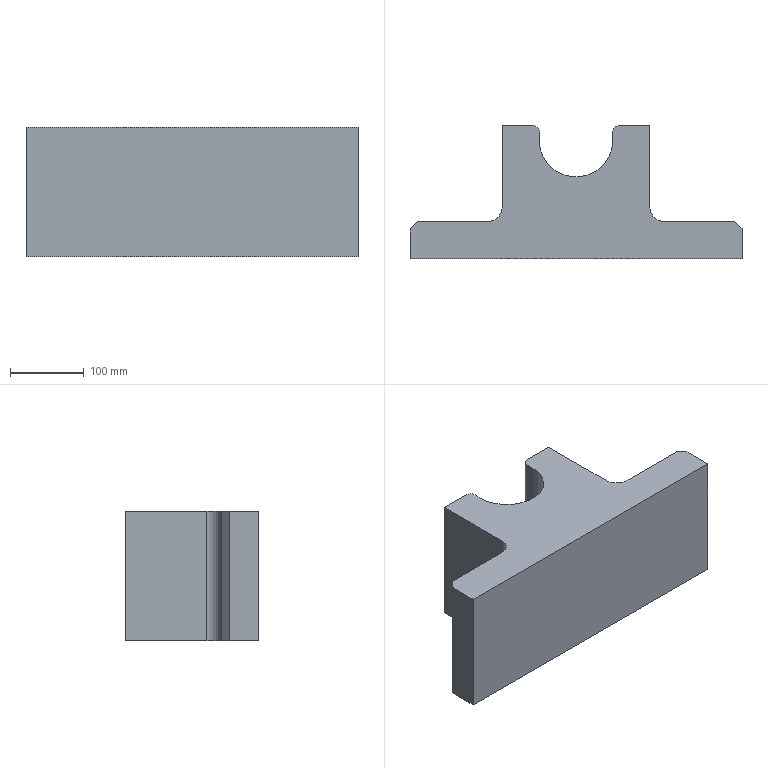Part | SolidWorks | features Fillet 2, Chamfer 1, Extrusion 1, ICE 1, MoveFace 1 | 1 solid | 21 faces | box 450 x 180.5 x 175 mm | volume 7476887 mm3 | plane 13 | cylinder 8 | commonest cylinder face diameters 20 x3 100 x3 40 x2
STEP:
#1=CARTESIAN_POINT('',(49.161,10.,87.5));
#2=VERTEX_POINT('',#1);
#3=CARTESIAN_POINT('',(49.301,8.333,87.5));
#4=VERTEX_POINT('',#3);
#5=CARTESIAN_POINT('',(59.161,10.,87.5));
#6=DIRECTION('',(0.,0.,1.));
#7=DIRECTION('',(1.,0.,0.));
#8=AXIS2_PLACEMENT_3D('',#5,#6,#7);
#9=CIRCLE('',#8,10.);
#10=EDGE_CURVE('',#2,#4,#9,.T.);
#11=ORIENTED_EDGE('',*,*,#10,.F.);
#12=CARTESIAN_POINT('',(49.161,10.,-87.5));
#13=VERTEX_POINT('',#12);
#14=CARTESIAN_POINT('',(49.161,10.,87.5));
#15=DIRECTION('',(0.,0.,-1.));
#16=VECTOR('',#15,1000.);
#17=LINE('',#14,#16);
#18=EDGE_CURVE('',#2,#13,#17,.T.);
#19=ORIENTED_EDGE('',*,*,#18,.T.);
#20=CARTESIAN_POINT('',(49.301,8.333,-87.5));
#21=VERTEX_POINT('',#20);
#22=CARTESIAN_POINT('',(59.161,10.,-87.5));
#23=DIRECTION('',(0.,0.,-1.));
#24=DIRECTION('',(1.,0.,0.));
#25=AXIS2_PLACEMENT_3D('',#22,#23,#24);
#26=CIRCLE('',#25,10.);
#27=EDGE_CURVE('',#21,#13,#26,.T.);
#28=ORIENTED_EDGE('',*,*,#27,.F.);
#29=CARTESIAN_POINT('',(49.301,8.333,87.5));
#30=DIRECTION('',(0.,0.,-1.));
#31=VECTOR('',#30,1000.);
#32=LINE('',#29,#31);
#33=EDGE_CURVE('',#4,#21,#32,.T.);
#34=ORIENTED_EDGE('',*,*,#33,.F.);
#35=EDGE_LOOP('',(#11,#19,#28,#34));
#36=FACE_OUTER_BOUND('',#35,.T.);
#37=CARTESIAN_POINT('',(59.161,10.,87.5));
#38=DIRECTION('',(0.,0.,-1.));
#39=DIRECTION('',(-1.,0.,0.));
#40=AXIS2_PLACEMENT_3D('',#37,#38,#39);
#41=CYLINDRICAL_SURFACE('',#40,10.);
#42=ADVANCED_FACE('',(#36),#41,.T.);
#43=CARTESIAN_POINT('',(-50.,0.,87.5));
#44=VERTEX_POINT('',#43);
#45=CARTESIAN_POINT('',(50.,0.,87.5));
#46=VERTEX_POINT('',#45);
#47=CARTESIAN_POINT('',(0.,0.,87.5));
#48=DIRECTION('',(0.,0.,1.));
#49=DIRECTION('',(1.,0.,0.));
#50=AXIS2_PLACEMENT_3D('',#47,#48,#49);
#51=CIRCLE('',#50,50.);
#52=EDGE_CURVE('',#44,#46,#51,.T.);
#53=ORIENTED_EDGE('',*,*,#52,.T.);
#54=CARTESIAN_POINT('',(50.,0.,-87.5));
#55=VERTEX_POINT('',#54);
#56=CARTESIAN_POINT('',(50.,0.,87.5));
#57=DIRECTION('',(0.,0.,-1.));
#58=VECTOR('',#57,1000.);
#59=LINE('',#56,#58);
#60=EDGE_CURVE('',#46,#55,#59,.T.);
#61=ORIENTED_EDGE('',*,*,#60,.T.);
#62=CARTESIAN_POINT('',(-50.,0.,-87.5));
#63=VERTEX_POINT('',#62);
#64=CARTESIAN_POINT('',(0.,0.,-87.5));
#65=DIRECTION('',(0.,0.,1.));
#66=DIRECTION('',(1.,0.,0.));
#67=AXIS2_PLACEMENT_3D('',#64,#65,#66);
#68=CIRCLE('',#67,50.);
#69=EDGE_CURVE('',#63,#55,#68,.T.);
#70=ORIENTED_EDGE('',*,*,#69,.F.);
#71=CARTESIAN_POINT('',(-50.,0.,87.5));
#72=DIRECTION('',(0.,0.,-1.));
#73=VECTOR('',#72,1000.);
#74=LINE('',#71,#73);
#75=EDGE_CURVE('',#44,#63,#74,.T.);
#76=ORIENTED_EDGE('',*,*,#75,.F.);
#77=EDGE_LOOP('',(#53,#61,#70,#76));
#78=FACE_OUTER_BOUND('',#77,.T.);
#79=CARTESIAN_POINT('',(0.,0.,87.5));
#80=DIRECTION('',(0.,0.,-1.));
#81=DIRECTION('',(-1.,0.,0.));
#82=AXIS2_PLACEMENT_3D('',#79,#80,#81);
#83=CYLINDRICAL_SURFACE('',#82,50.);
#84=ADVANCED_FACE('',(#78),#83,.F.);
#85=CARTESIAN_POINT('',(-49.301,8.333,87.5));
#86=VERTEX_POINT('',#85);
#87=CARTESIAN_POINT('',(0.,0.,87.5));
#88=DIRECTION('',(0.,0.,1.));
#89=DIRECTION('',(1.,0.,0.));
#90=AXIS2_PLACEMENT_3D('',#87,#88,#89);
#91=CIRCLE('',#90,50.);
#92=EDGE_CURVE('',#86,#44,#91,.T.);
#93=ORIENTED_EDGE('',*,*,#92,.T.);
#94=ORIENTED_EDGE('',*,*,#75,.T.);
#95=CARTESIAN_POINT('',(-49.301,8.333,-87.5));
#96=VERTEX_POINT('',#95);
#97=CARTESIAN_POINT('',(0.,0.,-87.5));
#98=DIRECTION('',(0.,0.,1.));
#99=DIRECTION('',(1.,0.,0.));
#100=AXIS2_PLACEMENT_3D('',#97,#98,#99);
#101=CIRCLE('',#100,50.);
#102=EDGE_CURVE('',#96,#63,#101,.T.);
#103=ORIENTED_EDGE('',*,*,#102,.F.);
#104=CARTESIAN_POINT('',(-49.301,8.333,87.5));
#105=DIRECTION('',(0.,0.,1.));
#106=VECTOR('',#105,1000.);
#107=LINE('',#104,#106);
#108=EDGE_CURVE('',#96,#86,#107,.T.);
#109=ORIENTED_EDGE('',*,*,#108,.T.);
#110=EDGE_LOOP('',(#93,#94,#103,#109));
#111=FACE_OUTER_BOUND('',#110,.T.);
#112=CARTESIAN_POINT('',(0.,0.,87.5));
#113=DIRECTION('',(0.,0.,-1.));
#114=DIRECTION('',(-1.,0.,0.));
#115=AXIS2_PLACEMENT_3D('',#112,#113,#114);
#116=CYLINDRICAL_SURFACE('',#115,50.);
#117=ADVANCED_FACE('',(#111),#116,.F.);
#118=ORIENTED_EDGE('',*,*,#60,.F.);
#119=CARTESIAN_POINT('',(0.,0.,87.5));
#120=DIRECTION('',(0.,0.,1.));
#121=DIRECTION('',(1.,0.,0.));
#122=AXIS2_PLACEMENT_3D('',#119,#120,#121);
#123=CIRCLE('',#122,50.);
#124=EDGE_CURVE('',#46,#4,#123,.T.);
#125=ORIENTED_EDGE('',*,*,#124,.T.);
#126=ORIENTED_EDGE('',*,*,#33,.T.);
#127=CARTESIAN_POINT('',(0.,0.,-87.5));
#128=DIRECTION('',(0.,0.,1.));
#129=DIRECTION('',(1.,0.,0.));
#130=AXIS2_PLACEMENT_3D('',#127,#128,#129);
#131=CIRCLE('',#130,50.);
#132=EDGE_CURVE('',#55,#21,#131,.T.);
#133=ORIENTED_EDGE('',*,*,#132,.F.);
#134=EDGE_LOOP('',(#118,#125,#126,#133));
#135=FACE_OUTER_BOUND('',#134,.T.);
#136=CARTESIAN_POINT('',(0.,0.,87.5));
#137=DIRECTION('',(0.,0.,-1.));
#138=DIRECTION('',(-1.,0.,0.));
#139=AXIS2_PLACEMENT_3D('',#136,#137,#138);
#140=CYLINDRICAL_SURFACE('',#139,50.);
#141=ADVANCED_FACE('',(#135),#140,.F.);
#142=CARTESIAN_POINT('',(225.,-120.5,87.5));
#143=VERTEX_POINT('',#142);
#144=CARTESIAN_POINT('',(225.,-160.5,87.5));
#145=VERTEX_POINT('',#144);
#146=CARTESIAN_POINT('',(225.,0.,87.5));
#147=DIRECTION('',(0.,-1.,0.));
#148=VECTOR('',#147,1000.);
#149=LINE('',#146,#148);
#150=EDGE_CURVE('',#143,#145,#149,.T.);
#151=ORIENTED_EDGE('',*,*,#150,.F.);
#152=CARTESIAN_POINT('',(215.,-110.5,87.5));
#153=VERTEX_POINT('',#152);
#154=CARTESIAN_POINT('',(52.25,52.25,87.5));
#155=DIRECTION('',(-0.7071,0.7071,0.));
#156=VECTOR('',#155,1000.);
#157=LINE('',#154,#156);
#158=EDGE_CURVE('',#143,#153,#157,.T.);
#159=ORIENTED_EDGE('',*,*,#158,.T.);
#160=CARTESIAN_POINT('',(120.,-110.5,87.5));
#161=VERTEX_POINT('',#160);
#162=CARTESIAN_POINT('',(0.,-110.5,87.5));
#163=DIRECTION('',(1.,0.,0.));
#164=VECTOR('',#163,1000.);
#165=LINE('',#162,#164);
#166=EDGE_CURVE('',#161,#153,#165,.T.);
#167=ORIENTED_EDGE('',*,*,#166,.F.);
#168=CARTESIAN_POINT('',(100.,-90.5,87.5));
#169=VERTEX_POINT('',#168);
#170=CARTESIAN_POINT('',(120.,-90.5,87.5));
#171=DIRECTION('',(0.,0.,-1.));
#172=DIRECTION('',(1.,0.,0.));
#173=AXIS2_PLACEMENT_3D('',#170,#171,#172);
#174=CIRCLE('',#173,20.);
#175=EDGE_CURVE('',#161,#169,#174,.T.);
#176=ORIENTED_EDGE('',*,*,#175,.T.);
#177=CARTESIAN_POINT('',(100.,20.,87.5));
#178=VERTEX_POINT('',#177);
#179=CARTESIAN_POINT('',(100.,0.,87.5));
#180=DIRECTION('',(0.,1.,0.));
#181=VECTOR('',#180,1000.);
#182=LINE('',#179,#181);
#183=EDGE_CURVE('',#169,#178,#182,.T.);
#184=ORIENTED_EDGE('',*,*,#183,.T.);
#185=CARTESIAN_POINT('',(59.161,20.,87.5));
#186=VERTEX_POINT('',#185);
#187=CARTESIAN_POINT('',(-100.,20.,87.5));
#188=DIRECTION('',(1.,0.,0.));
#189=VECTOR('',#188,1000.);
#190=LINE('',#187,#189);
#191=EDGE_CURVE('',#186,#178,#190,.T.);
#192=ORIENTED_EDGE('',*,*,#191,.F.);
#193=CARTESIAN_POINT('',(59.161,10.,87.5));
#194=DIRECTION('',(0.,0.,1.));
#195=DIRECTION('',(1.,0.,0.));
#196=AXIS2_PLACEMENT_3D('',#193,#194,#195);
#197=CIRCLE('',#196,10.);
#198=EDGE_CURVE('',#186,#2,#197,.T.);
#199=ORIENTED_EDGE('',*,*,#198,.T.);
#200=ORIENTED_EDGE('',*,*,#10,.T.);
#201=ORIENTED_EDGE('',*,*,#124,.F.);
#202=ORIENTED_EDGE('',*,*,#52,.F.);
#203=ORIENTED_EDGE('',*,*,#92,.F.);
#204=CARTESIAN_POINT('',(-59.161,20.,87.5));
#205=VERTEX_POINT('',#204);
#206=CARTESIAN_POINT('',(-59.161,10.,87.5));
#207=DIRECTION('',(0.,0.,1.));
#208=DIRECTION('',(1.,0.,0.));
#209=AXIS2_PLACEMENT_3D('',#206,#207,#208);
#210=CIRCLE('',#209,10.);
#211=EDGE_CURVE('',#86,#205,#210,.T.);
#212=ORIENTED_EDGE('',*,*,#211,.T.);
#213=CARTESIAN_POINT('',(-100.,20.,87.5));
#214=VERTEX_POINT('',#213);
#215=CARTESIAN_POINT('',(-100.,20.,87.5));
#216=DIRECTION('',(1.,0.,0.));
#217=VECTOR('',#216,1000.);
#218=LINE('',#215,#217);
#219=EDGE_CURVE('',#214,#205,#218,.T.);
#220=ORIENTED_EDGE('',*,*,#219,.F.);
#221=CARTESIAN_POINT('',(-100.,-90.5,87.5));
#222=VERTEX_POINT('',#221);
#223=CARTESIAN_POINT('',(-100.,0.,87.5));
#224=DIRECTION('',(0.,1.,0.));
#225=VECTOR('',#224,1000.);
#226=LINE('',#223,#225);
#227=EDGE_CURVE('',#222,#214,#226,.T.);
#228=ORIENTED_EDGE('',*,*,#227,.F.);
#229=CARTESIAN_POINT('',(-120.,-110.5,87.5));
#230=VERTEX_POINT('',#229);
#231=CARTESIAN_POINT('',(-120.,-90.5,87.5));
#232=DIRECTION('',(0.,0.,-1.));
#233=DIRECTION('',(1.,0.,0.));
#234=AXIS2_PLACEMENT_3D('',#231,#232,#233);
#235=CIRCLE('',#234,20.);
#236=EDGE_CURVE('',#222,#230,#235,.T.);
#237=ORIENTED_EDGE('',*,*,#236,.T.);
#238=CARTESIAN_POINT('',(-215.,-110.5,87.5));
#239=VERTEX_POINT('',#238);
#240=CARTESIAN_POINT('',(0.,-110.5,87.5));
#241=DIRECTION('',(1.,0.,0.));
#242=VECTOR('',#241,1000.);
#243=LINE('',#240,#242);
#244=EDGE_CURVE('',#239,#230,#243,.T.);
#245=ORIENTED_EDGE('',*,*,#244,.F.);
#246=CARTESIAN_POINT('',(-225.,-120.5,87.5));
#247=VERTEX_POINT('',#246);
#248=CARTESIAN_POINT('',(-52.25,52.25,87.5));
#249=DIRECTION('',(-0.7071,-0.7071,0.));
#250=VECTOR('',#249,1000.);
#251=LINE('',#248,#250);
#252=EDGE_CURVE('',#239,#247,#251,.T.);
#253=ORIENTED_EDGE('',*,*,#252,.T.);
#254=CARTESIAN_POINT('',(-225.,-160.5,87.5));
#255=VERTEX_POINT('',#254);
#256=CARTESIAN_POINT('',(-225.,0.,87.5));
#257=DIRECTION('',(0.,-1.,0.));
#258=VECTOR('',#257,1000.);
#259=LINE('',#256,#258);
#260=EDGE_CURVE('',#247,#255,#259,.T.);
#261=ORIENTED_EDGE('',*,*,#260,.T.);
#262=CARTESIAN_POINT('',(0.,-160.5,87.5));
#263=DIRECTION('',(1.,0.,0.));
#264=VECTOR('',#263,1000.);
#265=LINE('',#262,#264);
#266=EDGE_CURVE('',#255,#145,#265,.T.);
#267=ORIENTED_EDGE('',*,*,#266,.T.);
#268=EDGE_LOOP('',(#151,#159,#167,#176,#184,#192,#199,#200,#201,#202,#203,#212,#220,#228,#237,#245,#253,#261,#267));
#269=FACE_OUTER_BOUND('',#268,.T.);
#270=CARTESIAN_POINT('',(0.,0.,87.5));
#271=DIRECTION('',(0.,0.,1.));
#272=DIRECTION('',(1.,0.,0.));
#273=AXIS2_PLACEMENT_3D('',#270,#271,#272);
#274=PLANE('',#273);
#275=ADVANCED_FACE('',(#269),#274,.T.);
#276=CARTESIAN_POINT('',(120.,-110.5,-87.5));
#277=VERTEX_POINT('',#276);
#278=CARTESIAN_POINT('',(215.,-110.5,-87.5));
#279=VERTEX_POINT('',#278);
#280=CARTESIAN_POINT('',(0.,-110.5,-87.5));
#281=DIRECTION('',(1.,0.,0.));
#282=VECTOR('',#281,1000.);
#283=LINE('',#280,#282);
#284=EDGE_CURVE('',#277,#279,#283,.T.);
#285=ORIENTED_EDGE('',*,*,#284,.T.);
#286=CARTESIAN_POINT('',(225.,-120.5,-87.5));
#287=VERTEX_POINT('',#286);
#288=CARTESIAN_POINT('',(215.,-110.5,-87.5));
#289=DIRECTION('',(0.7071,-0.7071,0.));
#290=VECTOR('',#289,1000.);
#291=LINE('',#288,#290);
#292=EDGE_CURVE('',#279,#287,#291,.T.);
#293=ORIENTED_EDGE('',*,*,#292,.T.);
#294=CARTESIAN_POINT('',(225.,-160.5,-87.5));
#295=VERTEX_POINT('',#294);
#296=CARTESIAN_POINT('',(225.,0.,-87.5));
#297=DIRECTION('',(0.,-1.,0.));
#298=VECTOR('',#297,1000.);
#299=LINE('',#296,#298);
#300=EDGE_CURVE('',#287,#295,#299,.T.);
#301=ORIENTED_EDGE('',*,*,#300,.T.);
#302=CARTESIAN_POINT('',(-225.,-160.5,-87.5));
#303=VERTEX_POINT('',#302);
#304=CARTESIAN_POINT('',(0.,-160.5,-87.5));
#305=DIRECTION('',(1.,0.,0.));
#306=VECTOR('',#305,1000.);
#307=LINE('',#304,#306);
#308=EDGE_CURVE('',#303,#295,#307,.T.);
#309=ORIENTED_EDGE('',*,*,#308,.F.);
#310=CARTESIAN_POINT('',(-225.,-120.5,-87.5));
#311=VERTEX_POINT('',#310);
#312=CARTESIAN_POINT('',(-225.,0.,-87.5));
#313=DIRECTION('',(0.,-1.,0.));
#314=VECTOR('',#313,1000.);
#315=LINE('',#312,#314);
#316=EDGE_CURVE('',#311,#303,#315,.T.);
#317=ORIENTED_EDGE('',*,*,#316,.F.);
#318=CARTESIAN_POINT('',(-215.,-110.5,-87.5));
#319=VERTEX_POINT('',#318);
#320=CARTESIAN_POINT('',(-225.,-120.5,-87.5));
#321=DIRECTION('',(0.7071,0.7071,0.));
#322=VECTOR('',#321,1000.);
#323=LINE('',#320,#322);
#324=EDGE_CURVE('',#311,#319,#323,.T.);
#325=ORIENTED_EDGE('',*,*,#324,.T.);
#326=CARTESIAN_POINT('',(-120.,-110.5,-87.5));
#327=VERTEX_POINT('',#326);
#328=CARTESIAN_POINT('',(0.,-110.5,-87.5));
#329=DIRECTION('',(1.,0.,0.));
#330=VECTOR('',#329,1000.);
#331=LINE('',#328,#330);
#332=EDGE_CURVE('',#319,#327,#331,.T.);
#333=ORIENTED_EDGE('',*,*,#332,.T.);
#334=CARTESIAN_POINT('',(-100.,-90.5,-87.5));
#335=VERTEX_POINT('',#334);
#336=CARTESIAN_POINT('',(-120.,-90.5,-87.5));
#337=DIRECTION('',(0.,0.,1.));
#338=DIRECTION('',(1.,0.,0.));
#339=AXIS2_PLACEMENT_3D('',#336,#337,#338);
#340=CIRCLE('',#339,20.);
#341=EDGE_CURVE('',#327,#335,#340,.T.);
#342=ORIENTED_EDGE('',*,*,#341,.T.);
#343=CARTESIAN_POINT('',(-100.,20.,-87.5));
#344=VERTEX_POINT('',#343);
#345=CARTESIAN_POINT('',(-100.,0.,-87.5));
#346=DIRECTION('',(0.,1.,0.));
#347=VECTOR('',#346,1000.);
#348=LINE('',#345,#347);
#349=EDGE_CURVE('',#335,#344,#348,.T.);
#350=ORIENTED_EDGE('',*,*,#349,.T.);
#351=CARTESIAN_POINT('',(-59.161,20.,-87.5));
#352=VERTEX_POINT('',#351);
#353=CARTESIAN_POINT('',(0.,20.,-87.5));
#354=DIRECTION('',(-1.,0.,0.));
#355=VECTOR('',#354,1000.);
#356=LINE('',#353,#355);
#357=EDGE_CURVE('',#352,#344,#356,.T.);
#358=ORIENTED_EDGE('',*,*,#357,.F.);
#359=CARTESIAN_POINT('',(-59.161,10.,-87.5));
#360=DIRECTION('',(0.,0.,-1.));
#361=DIRECTION('',(1.,0.,0.));
#362=AXIS2_PLACEMENT_3D('',#359,#360,#361);
#363=CIRCLE('',#362,10.);
#364=EDGE_CURVE('',#352,#96,#363,.T.);
#365=ORIENTED_EDGE('',*,*,#364,.T.);
#366=ORIENTED_EDGE('',*,*,#102,.T.);
#367=ORIENTED_EDGE('',*,*,#69,.T.);
#368=ORIENTED_EDGE('',*,*,#132,.T.);
#369=ORIENTED_EDGE('',*,*,#27,.T.);
#370=CARTESIAN_POINT('',(59.161,20.,-87.5));
#371=VERTEX_POINT('',#370);
#372=CARTESIAN_POINT('',(59.161,10.,-87.5));
#373=DIRECTION('',(0.,0.,-1.));
#374=DIRECTION('',(1.,0.,0.));
#375=AXIS2_PLACEMENT_3D('',#372,#373,#374);
#376=CIRCLE('',#375,10.);
#377=EDGE_CURVE('',#13,#371,#376,.T.);
#378=ORIENTED_EDGE('',*,*,#377,.T.);
#379=CARTESIAN_POINT('',(100.,20.,-87.5));
#380=VERTEX_POINT('',#379);
#381=CARTESIAN_POINT('',(-100.,20.,-87.5));
#382=DIRECTION('',(-1.,0.,0.));
#383=VECTOR('',#382,1000.);
#384=LINE('',#381,#383);
#385=EDGE_CURVE('',#380,#371,#384,.T.);
#386=ORIENTED_EDGE('',*,*,#385,.F.);
#387=CARTESIAN_POINT('',(100.,-90.5,-87.5));
#388=VERTEX_POINT('',#387);
#389=CARTESIAN_POINT('',(100.,0.,-87.5));
#390=DIRECTION('',(0.,1.,0.));
#391=VECTOR('',#390,1000.);
#392=LINE('',#389,#391);
#393=EDGE_CURVE('',#388,#380,#392,.T.);
#394=ORIENTED_EDGE('',*,*,#393,.F.);
#395=CARTESIAN_POINT('',(120.,-90.5,-87.5));
#396=DIRECTION('',(0.,0.,1.));
#397=DIRECTION('',(1.,0.,0.));
#398=AXIS2_PLACEMENT_3D('',#395,#396,#397);
#399=CIRCLE('',#398,20.);
#400=EDGE_CURVE('',#388,#277,#399,.T.);
#401=ORIENTED_EDGE('',*,*,#400,.T.);
#402=EDGE_LOOP('',(#285,#293,#301,#309,#317,#325,#333,#342,#350,#358,#365,#366,#367,#368,#369,#378,#386,#394,#401));
#403=FACE_OUTER_BOUND('',#402,.T.);
#404=CARTESIAN_POINT('',(0.,0.,-87.5));
#405=DIRECTION('',(0.,0.,1.));
#406=DIRECTION('',(1.,0.,0.));
#407=AXIS2_PLACEMENT_3D('',#404,#405,#406);
#408=PLANE('',#407);
#409=ADVANCED_FACE('',(#403),#408,.F.);
#410=ORIENTED_EDGE('',*,*,#183,.F.);
#411=CARTESIAN_POINT('',(100.,-90.5,87.5));
#412=DIRECTION('',(0.,0.,-1.));
#413=VECTOR('',#412,1000.);
#414=LINE('',#411,#413);
#415=EDGE_CURVE('',#169,#388,#414,.T.);
#416=ORIENTED_EDGE('',*,*,#415,.T.);
#417=ORIENTED_EDGE('',*,*,#393,.T.);
#418=CARTESIAN_POINT('',(100.,20.,87.5));
#419=DIRECTION('',(0.,0.,-1.));
#420=VECTOR('',#419,1000.);
#421=LINE('',#418,#420);
#422=EDGE_CURVE('',#178,#380,#421,.T.);
#423=ORIENTED_EDGE('',*,*,#422,.F.);
#424=EDGE_LOOP('',(#410,#416,#417,#423));
#425=FACE_OUTER_BOUND('',#424,.T.);
#426=CARTESIAN_POINT('',(100.,0.,87.5));
#427=DIRECTION('',(-1.,0.,0.));
#428=DIRECTION('',(0.,-1.,0.));
#429=AXIS2_PLACEMENT_3D('',#426,#427,#428);
#430=PLANE('',#429);
#431=ADVANCED_FACE('',(#425),#430,.F.);
#432=ORIENTED_EDGE('',*,*,#349,.F.);
#433=CARTESIAN_POINT('',(-100.,-90.5,87.5));
#434=DIRECTION('',(0.,0.,1.));
#435=VECTOR('',#434,1000.);
#436=LINE('',#433,#435);
#437=EDGE_CURVE('',#335,#222,#436,.T.);
#438=ORIENTED_EDGE('',*,*,#437,.T.);
#439=ORIENTED_EDGE('',*,*,#227,.T.);
#440=CARTESIAN_POINT('',(-100.,20.,87.5));
#441=DIRECTION('',(0.,0.,-1.));
#442=VECTOR('',#441,1000.);
#443=LINE('',#440,#442);
#444=EDGE_CURVE('',#214,#344,#443,.T.);
#445=ORIENTED_EDGE('',*,*,#444,.T.);
#446=EDGE_LOOP('',(#432,#438,#439,#445));
#447=FACE_OUTER_BOUND('',#446,.T.);
#448=CARTESIAN_POINT('',(-100.,0.,87.5));
#449=DIRECTION('',(-1.,0.,0.));
#450=DIRECTION('',(0.,-1.,0.));
#451=AXIS2_PLACEMENT_3D('',#448,#449,#450);
#452=PLANE('',#451);
#453=ADVANCED_FACE('',(#447),#452,.T.);
#454=ORIENTED_EDGE('',*,*,#332,.F.);
#455=CARTESIAN_POINT('',(-215.,-110.5,87.5));
#456=DIRECTION('',(0.,0.,1.));
#457=VECTOR('',#456,1000.);
#458=LINE('',#455,#457);
#459=EDGE_CURVE('',#319,#239,#458,.T.);
#460=ORIENTED_EDGE('',*,*,#459,.T.);
#461=ORIENTED_EDGE('',*,*,#244,.T.);
#462=CARTESIAN_POINT('',(-120.,-110.5,-87.5));
#463=DIRECTION('',(0.,0.,-1.));
#464=VECTOR('',#463,1000.);
#465=LINE('',#462,#464);
#466=EDGE_CURVE('',#230,#327,#465,.T.);
#467=ORIENTED_EDGE('',*,*,#466,.T.);
#468=EDGE_LOOP('',(#454,#460,#461,#467));
#469=FACE_OUTER_BOUND('',#468,.T.);
#470=CARTESIAN_POINT('',(0.,-110.5,87.5));
#471=DIRECTION('',(0.,1.,0.));
#472=DIRECTION('',(-1.,0.,0.));
#473=AXIS2_PLACEMENT_3D('',#470,#471,#472);
#474=PLANE('',#473);
#475=ADVANCED_FACE('',(#469),#474,.T.);
#476=ORIENTED_EDGE('',*,*,#260,.F.);
#477=CARTESIAN_POINT('',(-225.,-120.5,-87.5));
#478=DIRECTION('',(0.,0.,-1.));
#479=VECTOR('',#478,1000.);
#480=LINE('',#477,#479);
#481=EDGE_CURVE('',#247,#311,#480,.T.);
#482=ORIENTED_EDGE('',*,*,#481,.T.);
#483=ORIENTED_EDGE('',*,*,#316,.T.);
#484=CARTESIAN_POINT('',(-225.,-160.5,87.5));
#485=DIRECTION('',(0.,0.,-1.));
#486=VECTOR('',#485,1000.);
#487=LINE('',#484,#486);
#488=EDGE_CURVE('',#255,#303,#487,.T.);
#489=ORIENTED_EDGE('',*,*,#488,.F.);
#490=EDGE_LOOP('',(#476,#482,#483,#489));
#491=FACE_OUTER_BOUND('',#490,.T.);
#492=CARTESIAN_POINT('',(-225.,0.,87.5));
#493=DIRECTION('',(1.,0.,0.));
#494=DIRECTION('',(0.,0.,-1.));
#495=AXIS2_PLACEMENT_3D('',#492,#493,#494);
#496=PLANE('',#495);
#497=ADVANCED_FACE('',(#491),#496,.F.);
#498=ORIENTED_EDGE('',*,*,#308,.T.);
#499=CARTESIAN_POINT('',(225.,-160.5,87.5));
#500=DIRECTION('',(0.,0.,-1.));
#501=VECTOR('',#500,1000.);
#502=LINE('',#499,#501);
#503=EDGE_CURVE('',#145,#295,#502,.T.);
#504=ORIENTED_EDGE('',*,*,#503,.F.);
#505=ORIENTED_EDGE('',*,*,#266,.F.);
#506=ORIENTED_EDGE('',*,*,#488,.T.);
#507=EDGE_LOOP('',(#498,#504,#505,#506));
#508=FACE_OUTER_BOUND('',#507,.T.);
#509=CARTESIAN_POINT('',(0.,-160.5,87.5));
#510=DIRECTION('',(0.,1.,0.));
#511=DIRECTION('',(-1.,0.,0.));
#512=AXIS2_PLACEMENT_3D('',#509,#510,#511);
#513=PLANE('',#512);
#514=ADVANCED_FACE('',(#508),#513,.F.);
#515=ORIENTED_EDGE('',*,*,#300,.F.);
#516=CARTESIAN_POINT('',(225.,-120.5,87.5));
#517=DIRECTION('',(0.,0.,1.));
#518=VECTOR('',#517,1000.);
#519=LINE('',#516,#518);
#520=EDGE_CURVE('',#287,#143,#519,.T.);
#521=ORIENTED_EDGE('',*,*,#520,.T.);
#522=ORIENTED_EDGE('',*,*,#150,.T.);
#523=ORIENTED_EDGE('',*,*,#503,.T.);
#524=EDGE_LOOP('',(#515,#521,#522,#523));
#525=FACE_OUTER_BOUND('',#524,.T.);
#526=CARTESIAN_POINT('',(225.,0.,87.5));
#527=DIRECTION('',(1.,0.,0.));
#528=DIRECTION('',(0.,1.,0.));
#529=AXIS2_PLACEMENT_3D('',#526,#527,#528);
#530=PLANE('',#529);
#531=ADVANCED_FACE('',(#525),#530,.T.);
#532=ORIENTED_EDGE('',*,*,#166,.T.);
#533=CARTESIAN_POINT('',(215.,-110.5,87.5));
#534=DIRECTION('',(0.,0.,-1.));
#535=VECTOR('',#534,1000.);
#536=LINE('',#533,#535);
#537=EDGE_CURVE('',#153,#279,#536,.T.);
#538=ORIENTED_EDGE('',*,*,#537,.T.);
#539=ORIENTED_EDGE('',*,*,#284,.F.);
#540=CARTESIAN_POINT('',(120.,-110.5,87.5));
#541=DIRECTION('',(0.,0.,1.));
#542=VECTOR('',#541,1000.);
#543=LINE('',#540,#542);
#544=EDGE_CURVE('',#277,#161,#543,.T.);
#545=ORIENTED_EDGE('',*,*,#544,.T.);
#546=EDGE_LOOP('',(#532,#538,#539,#545));
#547=FACE_OUTER_BOUND('',#546,.T.);
#548=CARTESIAN_POINT('',(0.,-110.5,87.5));
#549=DIRECTION('',(0.,1.,0.));
#550=DIRECTION('',(-1.,0.,0.));
#551=AXIS2_PLACEMENT_3D('',#548,#549,#550);
#552=PLANE('',#551);
#553=ADVANCED_FACE('',(#547),#552,.T.);
#554=ORIENTED_EDGE('',*,*,#219,.T.);
#555=CARTESIAN_POINT('',(-59.161,20.,0.));
#556=DIRECTION('',(0.,0.,-1.));
#557=VECTOR('',#556,1000.);
#558=LINE('',#555,#557);
#559=EDGE_CURVE('',#205,#352,#558,.T.);
#560=ORIENTED_EDGE('',*,*,#559,.T.);
#561=ORIENTED_EDGE('',*,*,#357,.T.);
#562=ORIENTED_EDGE('',*,*,#444,.F.);
#563=EDGE_LOOP('',(#554,#560,#561,#562));
#564=FACE_OUTER_BOUND('',#563,.T.);
#565=CARTESIAN_POINT('',(0.,20.,0.));
#566=DIRECTION('',(0.,1.,0.));
#567=DIRECTION('',(0.,0.,1.));
#568=AXIS2_PLACEMENT_3D('',#565,#566,#567);
#569=PLANE('',#568);
#570=ADVANCED_FACE('',(#564),#569,.T.);
#571=ORIENTED_EDGE('',*,*,#385,.T.);
#572=CARTESIAN_POINT('',(59.161,20.,0.));
#573=DIRECTION('',(0.,0.,1.));
#574=VECTOR('',#573,1000.);
#575=LINE('',#572,#574);
#576=EDGE_CURVE('',#371,#186,#575,.T.);
#577=ORIENTED_EDGE('',*,*,#576,.T.);
#578=ORIENTED_EDGE('',*,*,#191,.T.);
#579=ORIENTED_EDGE('',*,*,#422,.T.);
#580=EDGE_LOOP('',(#571,#577,#578,#579));
#581=FACE_OUTER_BOUND('',#580,.T.);
#582=CARTESIAN_POINT('',(0.,20.,0.));
#583=DIRECTION('',(0.,1.,0.));
#584=DIRECTION('',(0.,0.,1.));
#585=AXIS2_PLACEMENT_3D('',#582,#583,#584);
#586=PLANE('',#585);
#587=ADVANCED_FACE('',(#581),#586,.T.);
#588=ORIENTED_EDGE('',*,*,#18,.F.);
#589=ORIENTED_EDGE('',*,*,#198,.F.);
#590=ORIENTED_EDGE('',*,*,#576,.F.);
#591=ORIENTED_EDGE('',*,*,#377,.F.);
#592=EDGE_LOOP('',(#588,#589,#590,#591));
#593=FACE_OUTER_BOUND('',#592,.T.);
#594=CARTESIAN_POINT('',(59.161,10.,87.5));
#595=DIRECTION('',(0.,0.,-1.));
#596=DIRECTION('',(-1.,0.,0.));
#597=AXIS2_PLACEMENT_3D('',#594,#595,#596);
#598=CYLINDRICAL_SURFACE('',#597,10.);
#599=ADVANCED_FACE('',(#593),#598,.T.);
#600=ORIENTED_EDGE('',*,*,#364,.F.);
#601=ORIENTED_EDGE('',*,*,#559,.F.);
#602=ORIENTED_EDGE('',*,*,#211,.F.);
#603=ORIENTED_EDGE('',*,*,#108,.F.);
#604=EDGE_LOOP('',(#600,#601,#602,#603));
#605=FACE_OUTER_BOUND('',#604,.T.);
#606=CARTESIAN_POINT('',(-59.161,10.,87.5));
#607=DIRECTION('',(0.,0.,-1.));
#608=DIRECTION('',(-1.,0.,0.));
#609=AXIS2_PLACEMENT_3D('',#606,#607,#608);
#610=CYLINDRICAL_SURFACE('',#609,10.);
#611=ADVANCED_FACE('',(#605),#610,.T.);
#612=ORIENTED_EDGE('',*,*,#236,.F.);
#613=ORIENTED_EDGE('',*,*,#437,.F.);
#614=ORIENTED_EDGE('',*,*,#341,.F.);
#615=ORIENTED_EDGE('',*,*,#466,.F.);
#616=EDGE_LOOP('',(#612,#613,#614,#615));
#617=FACE_OUTER_BOUND('',#616,.T.);
#618=CARTESIAN_POINT('',(-120.,-90.5,87.5));
#619=DIRECTION('',(0.,0.,1.));
#620=DIRECTION('',(1.,0.,0.));
#621=AXIS2_PLACEMENT_3D('',#618,#619,#620);
#622=CYLINDRICAL_SURFACE('',#621,20.);
#623=ADVANCED_FACE('',(#617),#622,.F.);
#624=ORIENTED_EDGE('',*,*,#175,.F.);
#625=ORIENTED_EDGE('',*,*,#544,.F.);
#626=ORIENTED_EDGE('',*,*,#400,.F.);
#627=ORIENTED_EDGE('',*,*,#415,.F.);
#628=EDGE_LOOP('',(#624,#625,#626,#627));
#629=FACE_OUTER_BOUND('',#628,.T.);
#630=CARTESIAN_POINT('',(120.,-90.5,87.5));
#631=DIRECTION('',(0.,0.,-1.));
#632=DIRECTION('',(-1.,0.,0.));
#633=AXIS2_PLACEMENT_3D('',#630,#631,#632);
#634=CYLINDRICAL_SURFACE('',#633,20.);
#635=ADVANCED_FACE('',(#629),#634,.F.);
#636=ORIENTED_EDGE('',*,*,#158,.F.);
#637=ORIENTED_EDGE('',*,*,#520,.F.);
#638=ORIENTED_EDGE('',*,*,#292,.F.);
#639=ORIENTED_EDGE('',*,*,#537,.F.);
#640=EDGE_LOOP('',(#636,#637,#638,#639));
#641=FACE_OUTER_BOUND('',#640,.T.);
#642=CARTESIAN_POINT('',(215.,-110.5,87.5));
#643=DIRECTION('',(-0.7071,-0.7071,0.));
#644=DIRECTION('',(0.,0.,-1.));
#645=AXIS2_PLACEMENT_3D('',#642,#643,#644);
#646=PLANE('',#645);
#647=ADVANCED_FACE('',(#641),#646,.F.);
#648=ORIENTED_EDGE('',*,*,#252,.F.);
#649=ORIENTED_EDGE('',*,*,#459,.F.);
#650=ORIENTED_EDGE('',*,*,#324,.F.);
#651=ORIENTED_EDGE('',*,*,#481,.F.);
#652=EDGE_LOOP('',(#648,#649,#650,#651));
#653=FACE_OUTER_BOUND('',#652,.T.);
#654=CARTESIAN_POINT('',(-225.,-120.5,87.5));
#655=DIRECTION('',(-0.7071,0.7071,0.));
#656=DIRECTION('',(0.,0.,1.));
#657=AXIS2_PLACEMENT_3D('',#654,#655,#656);
#658=PLANE('',#657);
#659=ADVANCED_FACE('',(#653),#658,.T.);
#660=CLOSED_SHELL('',(#42,#84,#117,#141,#275,#409,#431,#453,#475,#497,#514,#531,#553,#570,#587,#599,#611,#623,#635,#647,#659));
#661=MANIFOLD_SOLID_BREP('',#660);
#662=CARTESIAN_POINT('',(0.,0.,0.));
#663=DIRECTION('',(0.,0.,1.));
#664=DIRECTION('',(1.,0.,0.));
#665=AXIS2_PLACEMENT_3D('',#662,#663,#664);
#666=(LENGTH_UNIT()NAMED_UNIT(*)SI_UNIT(.MILLI.,.METRE.));
#667=UNCERTAINTY_MEASURE_WITH_UNIT(LENGTH_MEASURE(0.00001),#666,'','');
#668=(NAMED_UNIT(*)PLANE_ANGLE_UNIT()SI_UNIT($,.RADIAN.));
#669=(NAMED_UNIT(*)SI_UNIT($,.STERADIAN.)SOLID_ANGLE_UNIT());
#670=(GEOMETRIC_REPRESENTATION_CONTEXT(3)GLOBAL_UNCERTAINTY_ASSIGNED_CONTEXT((#667))GLOBAL_UNIT_ASSIGNED_CONTEXT((#666,#668,#669))REPRESENTATION_CONTEXT('',''));
#671=ADVANCED_BREP_SHAPE_REPRESENTATION('',(#661,#665),#670);